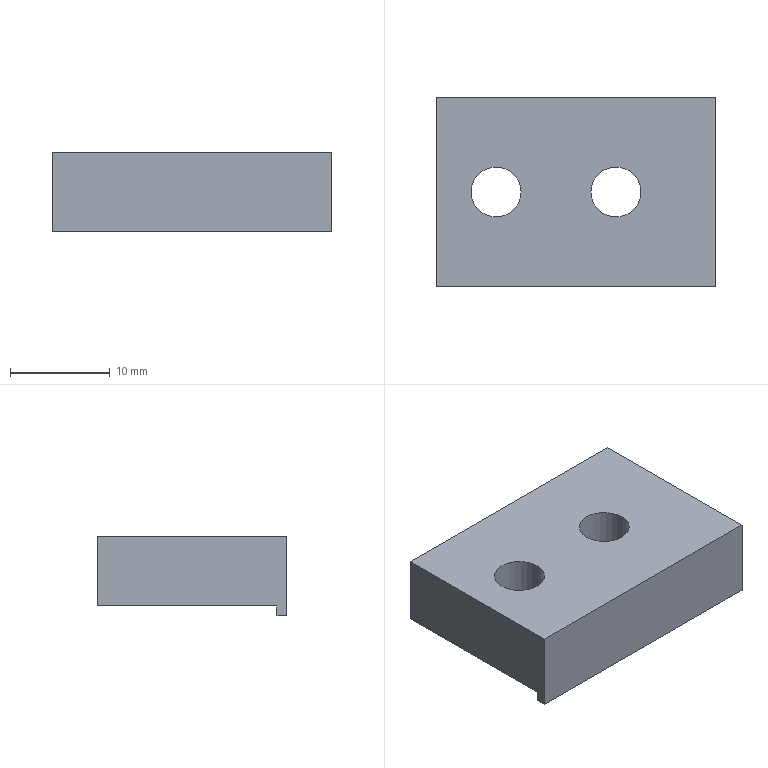Part | NX | 1 solid | 12 faces | box 28 x 19 x 8 mm | volume 3477 mm3 | plane 8 | cylinder 4 | commonest cylinder face diameters 5 x4
STEP:
#1=CARTESIAN_POINT('',(28.,0.,0.));
#2=VERTEX_POINT('',#1);
#3=CARTESIAN_POINT('',(28.,-18.,0.));
#4=VERTEX_POINT('',#3);
#5=CARTESIAN_POINT('',(28.,0.,0.));
#6=DIRECTION('',(0.,-1.,0.));
#7=VECTOR('',#6,1000.);
#8=LINE('',#5,#7);
#9=EDGE_CURVE('',#2,#4,#8,.T.);
#10=ORIENTED_EDGE('',*,*,#9,.T.);
#11=CARTESIAN_POINT('',(0.,-18.,0.));
#12=VERTEX_POINT('',#11);
#13=CARTESIAN_POINT('',(28.,-18.,0.));
#14=DIRECTION('',(-1.,0.,0.));
#15=VECTOR('',#14,1000.);
#16=LINE('',#13,#15);
#17=EDGE_CURVE('',#4,#12,#16,.T.);
#18=ORIENTED_EDGE('',*,*,#17,.T.);
#19=CARTESIAN_POINT('',(0.,0.,0.));
#20=VERTEX_POINT('',#19);
#21=CARTESIAN_POINT('',(0.,-18.,0.));
#22=DIRECTION('',(0.,1.,0.));
#23=VECTOR('',#22,1000.);
#24=LINE('',#21,#23);
#25=EDGE_CURVE('',#12,#20,#24,.T.);
#26=ORIENTED_EDGE('',*,*,#25,.T.);
#27=CARTESIAN_POINT('',(0.,0.,0.));
#28=DIRECTION('',(1.,0.,0.));
#29=VECTOR('',#28,1000.);
#30=LINE('',#27,#29);
#31=EDGE_CURVE('',#20,#2,#30,.T.);
#32=ORIENTED_EDGE('',*,*,#31,.T.);
#33=EDGE_LOOP('',(#10,#18,#26,#32));
#34=FACE_BOUND('',#33,.T.);
#35=CARTESIAN_POINT('',(8.5,-9.5,0.));
#36=VERTEX_POINT('',#35);
#37=CARTESIAN_POINT('',(3.5,-9.5,0.));
#38=VERTEX_POINT('',#37);
#39=CARTESIAN_POINT('',(6.,-9.5,0.));
#40=DIRECTION('',(0.,0.,-1.));
#41=DIRECTION('',(1.,0.,0.));
#42=AXIS2_PLACEMENT_3D('',#39,#40,#41);
#43=CIRCLE('',#42,2.5);
#44=EDGE_CURVE('',#36,#38,#43,.T.);
#45=ORIENTED_EDGE('',*,*,#44,.F.);
#46=CARTESIAN_POINT('',(6.,-9.5,0.));
#47=DIRECTION('',(0.,0.,-1.));
#48=DIRECTION('',(1.,0.,0.));
#49=AXIS2_PLACEMENT_3D('',#46,#47,#48);
#50=CIRCLE('',#49,2.5);
#51=EDGE_CURVE('',#38,#36,#50,.T.);
#52=ORIENTED_EDGE('',*,*,#51,.F.);
#53=EDGE_LOOP('',(#45,#52));
#54=FACE_BOUND('',#53,.T.);
#55=CARTESIAN_POINT('',(20.5,-9.5,0.));
#56=VERTEX_POINT('',#55);
#57=CARTESIAN_POINT('',(15.5,-9.5,0.));
#58=VERTEX_POINT('',#57);
#59=CARTESIAN_POINT('',(18.,-9.5,0.));
#60=DIRECTION('',(0.,0.,-1.));
#61=DIRECTION('',(1.,0.,0.));
#62=AXIS2_PLACEMENT_3D('',#59,#60,#61);
#63=CIRCLE('',#62,2.5);
#64=EDGE_CURVE('',#56,#58,#63,.T.);
#65=ORIENTED_EDGE('',*,*,#64,.F.);
#66=CARTESIAN_POINT('',(18.,-9.5,0.));
#67=DIRECTION('',(0.,0.,-1.));
#68=DIRECTION('',(1.,0.,0.));
#69=AXIS2_PLACEMENT_3D('',#66,#67,#68);
#70=CIRCLE('',#69,2.5);
#71=EDGE_CURVE('',#58,#56,#70,.T.);
#72=ORIENTED_EDGE('',*,*,#71,.F.);
#73=EDGE_LOOP('',(#65,#72));
#74=FACE_BOUND('',#73,.T.);
#75=CARTESIAN_POINT('',(0.,0.,0.));
#76=DIRECTION('',(0.,0.,1.));
#77=DIRECTION('',(1.,0.,0.));
#78=AXIS2_PLACEMENT_3D('',#75,#76,#77);
#79=PLANE('',#78);
#80=ADVANCED_FACE('',(#34,#54,#74),#79,.F.);
#81=ORIENTED_EDGE('',*,*,#9,.F.);
#82=CARTESIAN_POINT('',(28.,0.,7.));
#83=VERTEX_POINT('',#82);
#84=CARTESIAN_POINT('',(28.,0.,7.));
#85=DIRECTION('',(0.,0.,-1.));
#86=VECTOR('',#85,1000.);
#87=LINE('',#84,#86);
#88=EDGE_CURVE('',#83,#2,#87,.T.);
#89=ORIENTED_EDGE('',*,*,#88,.F.);
#90=CARTESIAN_POINT('',(28.,-19.,7.));
#91=VERTEX_POINT('',#90);
#92=CARTESIAN_POINT('',(28.,0.,7.));
#93=DIRECTION('',(0.,-1.,0.));
#94=VECTOR('',#93,1000.);
#95=LINE('',#92,#94);
#96=EDGE_CURVE('',#83,#91,#95,.T.);
#97=ORIENTED_EDGE('',*,*,#96,.T.);
#98=CARTESIAN_POINT('',(28.,-19.,-1.));
#99=VERTEX_POINT('',#98);
#100=CARTESIAN_POINT('',(28.,-19.,7.));
#101=DIRECTION('',(0.,0.,-1.));
#102=VECTOR('',#101,1000.);
#103=LINE('',#100,#102);
#104=EDGE_CURVE('',#91,#99,#103,.T.);
#105=ORIENTED_EDGE('',*,*,#104,.T.);
#106=CARTESIAN_POINT('',(28.,-18.,-1.));
#107=VERTEX_POINT('',#106);
#108=CARTESIAN_POINT('',(28.,-19.,-1.));
#109=DIRECTION('',(0.,1.,0.));
#110=VECTOR('',#109,1000.);
#111=LINE('',#108,#110);
#112=EDGE_CURVE('',#99,#107,#111,.T.);
#113=ORIENTED_EDGE('',*,*,#112,.T.);
#114=CARTESIAN_POINT('',(28.,-18.,0.));
#115=DIRECTION('',(0.,0.,-1.));
#116=VECTOR('',#115,1000.);
#117=LINE('',#114,#116);
#118=EDGE_CURVE('',#4,#107,#117,.T.);
#119=ORIENTED_EDGE('',*,*,#118,.F.);
#120=EDGE_LOOP('',(#81,#89,#97,#105,#113,#119));
#121=FACE_BOUND('',#120,.T.);
#122=CARTESIAN_POINT('',(28.,-18.,0.));
#123=DIRECTION('',(1.,0.,0.));
#124=DIRECTION('',(0.,1.,0.));
#125=AXIS2_PLACEMENT_3D('',#122,#123,#124);
#126=PLANE('',#125);
#127=ADVANCED_FACE('',(#121),#126,.T.);
#128=ORIENTED_EDGE('',*,*,#17,.F.);
#129=ORIENTED_EDGE('',*,*,#118,.T.);
#130=CARTESIAN_POINT('',(0.,-18.,-1.));
#131=VERTEX_POINT('',#130);
#132=CARTESIAN_POINT('',(28.,-18.,-1.));
#133=DIRECTION('',(-1.,0.,0.));
#134=VECTOR('',#133,1000.);
#135=LINE('',#132,#134);
#136=EDGE_CURVE('',#107,#131,#135,.T.);
#137=ORIENTED_EDGE('',*,*,#136,.T.);
#138=CARTESIAN_POINT('',(0.,-18.,-1.));
#139=DIRECTION('',(0.,0.,1.));
#140=VECTOR('',#139,1000.);
#141=LINE('',#138,#140);
#142=EDGE_CURVE('',#131,#12,#141,.T.);
#143=ORIENTED_EDGE('',*,*,#142,.T.);
#144=EDGE_LOOP('',(#128,#129,#137,#143));
#145=FACE_BOUND('',#144,.T.);
#146=CARTESIAN_POINT('',(0.,-18.,0.));
#147=DIRECTION('',(0.,-1.,0.));
#148=DIRECTION('',(0.,0.,-1.));
#149=AXIS2_PLACEMENT_3D('',#146,#147,#148);
#150=PLANE('',#149);
#151=ADVANCED_FACE('',(#145),#150,.F.);
#152=CARTESIAN_POINT('',(0.,-19.,7.));
#153=VERTEX_POINT('',#152);
#154=CARTESIAN_POINT('',(0.,0.,7.));
#155=VERTEX_POINT('',#154);
#156=CARTESIAN_POINT('',(0.,-19.,7.));
#157=DIRECTION('',(0.,1.,0.));
#158=VECTOR('',#157,1000.);
#159=LINE('',#156,#158);
#160=EDGE_CURVE('',#153,#155,#159,.T.);
#161=ORIENTED_EDGE('',*,*,#160,.T.);
#162=CARTESIAN_POINT('',(0.,0.,7.));
#163=DIRECTION('',(0.,0.,-1.));
#164=VECTOR('',#163,1000.);
#165=LINE('',#162,#164);
#166=EDGE_CURVE('',#155,#20,#165,.T.);
#167=ORIENTED_EDGE('',*,*,#166,.T.);
#168=ORIENTED_EDGE('',*,*,#25,.F.);
#169=ORIENTED_EDGE('',*,*,#142,.F.);
#170=CARTESIAN_POINT('',(0.,-19.,-1.));
#171=VERTEX_POINT('',#170);
#172=CARTESIAN_POINT('',(0.,-19.,-1.));
#173=DIRECTION('',(0.,1.,0.));
#174=VECTOR('',#173,1000.);
#175=LINE('',#172,#174);
#176=EDGE_CURVE('',#171,#131,#175,.T.);
#177=ORIENTED_EDGE('',*,*,#176,.F.);
#178=CARTESIAN_POINT('',(0.,-19.,-1.));
#179=DIRECTION('',(0.,0.,1.));
#180=VECTOR('',#179,1000.);
#181=LINE('',#178,#180);
#182=EDGE_CURVE('',#171,#153,#181,.T.);
#183=ORIENTED_EDGE('',*,*,#182,.T.);
#184=EDGE_LOOP('',(#161,#167,#168,#169,#177,#183));
#185=FACE_BOUND('',#184,.T.);
#186=CARTESIAN_POINT('',(0.,0.,0.));
#187=DIRECTION('',(-1.,0.,0.));
#188=DIRECTION('',(0.,0.,1.));
#189=AXIS2_PLACEMENT_3D('',#186,#187,#188);
#190=PLANE('',#189);
#191=ADVANCED_FACE('',(#185),#190,.T.);
#192=ORIENTED_EDGE('',*,*,#96,.F.);
#193=CARTESIAN_POINT('',(0.,0.,7.));
#194=DIRECTION('',(1.,0.,0.));
#195=VECTOR('',#194,1000.);
#196=LINE('',#193,#195);
#197=EDGE_CURVE('',#155,#83,#196,.T.);
#198=ORIENTED_EDGE('',*,*,#197,.F.);
#199=ORIENTED_EDGE('',*,*,#160,.F.);
#200=CARTESIAN_POINT('',(0.,-19.,7.));
#201=DIRECTION('',(1.,0.,0.));
#202=VECTOR('',#201,1000.);
#203=LINE('',#200,#202);
#204=EDGE_CURVE('',#153,#91,#203,.T.);
#205=ORIENTED_EDGE('',*,*,#204,.T.);
#206=EDGE_LOOP('',(#192,#198,#199,#205));
#207=FACE_BOUND('',#206,.T.);
#208=CARTESIAN_POINT('',(3.5,-9.5,7.));
#209=VERTEX_POINT('',#208);
#210=CARTESIAN_POINT('',(8.5,-9.5,7.));
#211=VERTEX_POINT('',#210);
#212=CARTESIAN_POINT('',(6.,-9.5,7.));
#213=DIRECTION('',(0.,0.,1.));
#214=DIRECTION('',(-1.,0.,0.));
#215=AXIS2_PLACEMENT_3D('',#212,#213,#214);
#216=CIRCLE('',#215,2.5);
#217=EDGE_CURVE('',#209,#211,#216,.T.);
#218=ORIENTED_EDGE('',*,*,#217,.F.);
#219=CARTESIAN_POINT('',(6.,-9.5,7.));
#220=DIRECTION('',(0.,0.,1.));
#221=DIRECTION('',(-1.,0.,0.));
#222=AXIS2_PLACEMENT_3D('',#219,#220,#221);
#223=CIRCLE('',#222,2.5);
#224=EDGE_CURVE('',#211,#209,#223,.T.);
#225=ORIENTED_EDGE('',*,*,#224,.F.);
#226=EDGE_LOOP('',(#218,#225));
#227=FACE_BOUND('',#226,.T.);
#228=CARTESIAN_POINT('',(15.5,-9.5,7.));
#229=VERTEX_POINT('',#228);
#230=CARTESIAN_POINT('',(20.5,-9.5,7.));
#231=VERTEX_POINT('',#230);
#232=CARTESIAN_POINT('',(18.,-9.5,7.));
#233=DIRECTION('',(0.,0.,1.));
#234=DIRECTION('',(-1.,0.,0.));
#235=AXIS2_PLACEMENT_3D('',#232,#233,#234);
#236=CIRCLE('',#235,2.5);
#237=EDGE_CURVE('',#229,#231,#236,.T.);
#238=ORIENTED_EDGE('',*,*,#237,.F.);
#239=CARTESIAN_POINT('',(18.,-9.5,7.));
#240=DIRECTION('',(0.,0.,1.));
#241=DIRECTION('',(-1.,0.,0.));
#242=AXIS2_PLACEMENT_3D('',#239,#240,#241);
#243=CIRCLE('',#242,2.5);
#244=EDGE_CURVE('',#231,#229,#243,.T.);
#245=ORIENTED_EDGE('',*,*,#244,.F.);
#246=EDGE_LOOP('',(#238,#245));
#247=FACE_BOUND('',#246,.T.);
#248=CARTESIAN_POINT('',(0.,0.,7.));
#249=DIRECTION('',(0.,0.,1.));
#250=DIRECTION('',(1.,0.,0.));
#251=AXIS2_PLACEMENT_3D('',#248,#249,#250);
#252=PLANE('',#251);
#253=ADVANCED_FACE('',(#207,#227,#247),#252,.T.);
#254=ORIENTED_EDGE('',*,*,#204,.F.);
#255=ORIENTED_EDGE('',*,*,#182,.F.);
#256=CARTESIAN_POINT('',(28.,-19.,-1.));
#257=DIRECTION('',(-1.,0.,0.));
#258=VECTOR('',#257,1000.);
#259=LINE('',#256,#258);
#260=EDGE_CURVE('',#99,#171,#259,.T.);
#261=ORIENTED_EDGE('',*,*,#260,.F.);
#262=ORIENTED_EDGE('',*,*,#104,.F.);
#263=EDGE_LOOP('',(#254,#255,#261,#262));
#264=FACE_BOUND('',#263,.T.);
#265=CARTESIAN_POINT('',(0.,-19.,0.));
#266=DIRECTION('',(0.,-1.,0.));
#267=DIRECTION('',(0.,0.,-1.));
#268=AXIS2_PLACEMENT_3D('',#265,#266,#267);
#269=PLANE('',#268);
#270=ADVANCED_FACE('',(#264),#269,.T.);
#271=ORIENTED_EDGE('',*,*,#136,.F.);
#272=ORIENTED_EDGE('',*,*,#112,.F.);
#273=ORIENTED_EDGE('',*,*,#260,.T.);
#274=ORIENTED_EDGE('',*,*,#176,.T.);
#275=EDGE_LOOP('',(#271,#272,#273,#274));
#276=FACE_BOUND('',#275,.T.);
#277=CARTESIAN_POINT('',(0.,-18.,-1.));
#278=DIRECTION('',(0.,0.,-1.));
#279=DIRECTION('',(0.,-1.,0.));
#280=AXIS2_PLACEMENT_3D('',#277,#278,#279);
#281=PLANE('',#280);
#282=ADVANCED_FACE('',(#276),#281,.T.);
#283=ORIENTED_EDGE('',*,*,#31,.F.);
#284=ORIENTED_EDGE('',*,*,#166,.F.);
#285=ORIENTED_EDGE('',*,*,#197,.T.);
#286=ORIENTED_EDGE('',*,*,#88,.T.);
#287=EDGE_LOOP('',(#283,#284,#285,#286));
#288=FACE_BOUND('',#287,.T.);
#289=CARTESIAN_POINT('',(28.,0.,0.));
#290=DIRECTION('',(0.,1.,0.));
#291=DIRECTION('',(1.,0.,0.));
#292=AXIS2_PLACEMENT_3D('',#289,#290,#291);
#293=PLANE('',#292);
#294=ADVANCED_FACE('',(#288),#293,.T.);
#295=ORIENTED_EDGE('',*,*,#44,.T.);
#296=CARTESIAN_POINT('',(3.5,-9.5,7.));
#297=DIRECTION('',(0.,0.,-1.));
#298=VECTOR('',#297,1000.);
#299=LINE('',#296,#298);
#300=EDGE_CURVE('',#38,#209,#299,.F.);
#301=ORIENTED_EDGE('',*,*,#300,.T.);
#302=ORIENTED_EDGE('',*,*,#217,.T.);
#303=CARTESIAN_POINT('',(8.5,-9.5,7.));
#304=DIRECTION('',(0.,0.,-1.));
#305=VECTOR('',#304,1000.);
#306=LINE('',#303,#305);
#307=EDGE_CURVE('',#36,#211,#306,.F.);
#308=ORIENTED_EDGE('',*,*,#307,.F.);
#309=EDGE_LOOP('',(#295,#301,#302,#308));
#310=FACE_BOUND('',#309,.T.);
#311=CARTESIAN_POINT('',(6.,-9.5,7.));
#312=DIRECTION('',(0.,0.,-1.));
#313=DIRECTION('',(-1.,0.,0.));
#314=AXIS2_PLACEMENT_3D('',#311,#312,#313);
#315=CYLINDRICAL_SURFACE('',#314,2.5);
#316=ADVANCED_FACE('',(#310),#315,.F.);
#317=ORIENTED_EDGE('',*,*,#64,.T.);
#318=CARTESIAN_POINT('',(15.5,-9.5,7.));
#319=DIRECTION('',(0.,0.,-1.));
#320=VECTOR('',#319,1000.);
#321=LINE('',#318,#320);
#322=EDGE_CURVE('',#58,#229,#321,.F.);
#323=ORIENTED_EDGE('',*,*,#322,.T.);
#324=ORIENTED_EDGE('',*,*,#237,.T.);
#325=CARTESIAN_POINT('',(20.5,-9.5,7.));
#326=DIRECTION('',(0.,0.,-1.));
#327=VECTOR('',#326,1000.);
#328=LINE('',#325,#327);
#329=EDGE_CURVE('',#56,#231,#328,.F.);
#330=ORIENTED_EDGE('',*,*,#329,.F.);
#331=EDGE_LOOP('',(#317,#323,#324,#330));
#332=FACE_BOUND('',#331,.T.);
#333=CARTESIAN_POINT('',(18.,-9.5,7.));
#334=DIRECTION('',(0.,0.,-1.));
#335=DIRECTION('',(-1.,0.,0.));
#336=AXIS2_PLACEMENT_3D('',#333,#334,#335);
#337=CYLINDRICAL_SURFACE('',#336,2.5);
#338=ADVANCED_FACE('',(#332),#337,.F.);
#339=ORIENTED_EDGE('',*,*,#322,.F.);
#340=ORIENTED_EDGE('',*,*,#71,.T.);
#341=ORIENTED_EDGE('',*,*,#329,.T.);
#342=ORIENTED_EDGE('',*,*,#244,.T.);
#343=EDGE_LOOP('',(#339,#340,#341,#342));
#344=FACE_BOUND('',#343,.T.);
#345=CARTESIAN_POINT('',(18.,-9.5,7.));
#346=DIRECTION('',(0.,0.,-1.));
#347=DIRECTION('',(-1.,0.,0.));
#348=AXIS2_PLACEMENT_3D('',#345,#346,#347);
#349=CYLINDRICAL_SURFACE('',#348,2.5);
#350=ADVANCED_FACE('',(#344),#349,.F.);
#351=ORIENTED_EDGE('',*,*,#300,.F.);
#352=ORIENTED_EDGE('',*,*,#51,.T.);
#353=ORIENTED_EDGE('',*,*,#307,.T.);
#354=ORIENTED_EDGE('',*,*,#224,.T.);
#355=EDGE_LOOP('',(#351,#352,#353,#354));
#356=FACE_BOUND('',#355,.T.);
#357=CARTESIAN_POINT('',(6.,-9.5,7.));
#358=DIRECTION('',(0.,0.,-1.));
#359=DIRECTION('',(-1.,0.,0.));
#360=AXIS2_PLACEMENT_3D('',#357,#358,#359);
#361=CYLINDRICAL_SURFACE('',#360,2.5);
#362=ADVANCED_FACE('',(#356),#361,.F.);
#363=CLOSED_SHELL('',(#80,#127,#151,#191,#253,#270,#282,#294,#316,#338,#350,#362));
#364=MANIFOLD_SOLID_BREP('',#363);
#365=(LENGTH_UNIT()NAMED_UNIT(*)SI_UNIT(.MILLI.,.METRE.));
#366=UNCERTAINTY_MEASURE_WITH_UNIT(LENGTH_MEASURE(0.00001),#365,'','');
#367=(NAMED_UNIT(*)PLANE_ANGLE_UNIT()SI_UNIT($,.RADIAN.));
#368=(NAMED_UNIT(*)SI_UNIT($,.STERADIAN.)SOLID_ANGLE_UNIT());
#369=(GEOMETRIC_REPRESENTATION_CONTEXT(3)GLOBAL_UNCERTAINTY_ASSIGNED_CONTEXT((#366))GLOBAL_UNIT_ASSIGNED_CONTEXT((#365,#367,#368))REPRESENTATION_CONTEXT('',''));
#370=ADVANCED_BREP_SHAPE_REPRESENTATION('',(#364),#369);